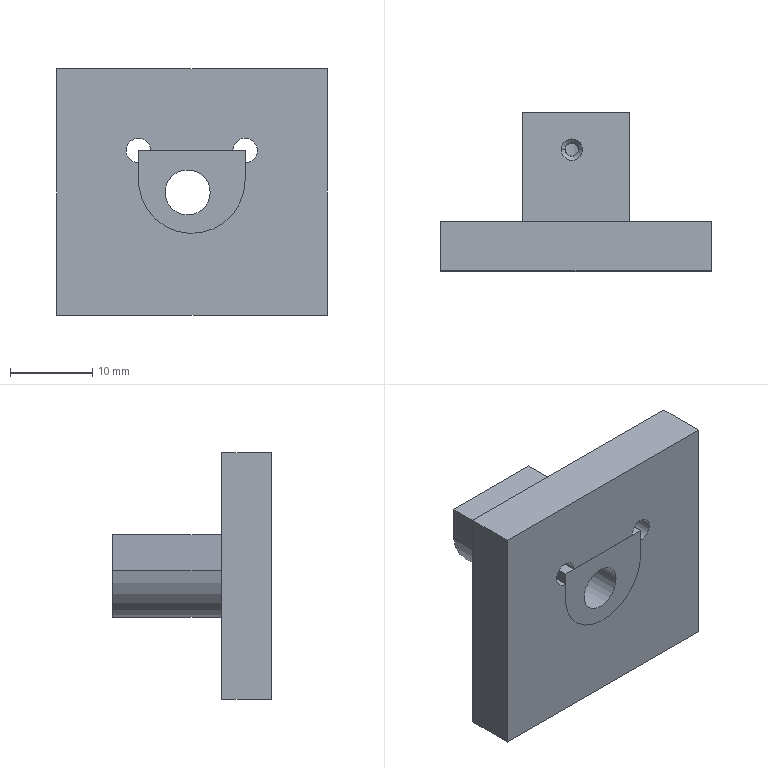NC program | NX | posted with a generic post | part box 32.951 x 19.3 x 30.1 mm
Lines 41 to 897 of 2866:
(ZLEVEL_PROFILE_COPY_1 , TOOL : D6)
N68 T06 M6
N70 G54
N72 G17 G0 G90 X-9.554 Y-0.868 B0. C0. S9500 M3
N74 G43 Z30. H6
N76 Z1.5
N78 G94 G1 X-9.55 Y-0.467 Z1.479 F1000.
N80 X-9.505 Y-0.031 Z1.456
N82 X-9.275 Y1.064 Z1.397
N84 X-8.921 Y2.124 Z1.339
N86 X-8.445 Y3.136 Z1.28
N88 X-7.855 Y4.086 Z1.222
N90 X-7.159 Y4.961 Z1.163
N92 X-6.365 Y5.75 Z1.104
N94 X-5.486 Y6.44 Z1.046
N96 X-4.532 Y7.024 Z0.987
N98 X-3.741 Y7.402 Z0.941
N100 X-2.577 Y7.808 Z0.877
N102 X-1.371 Y8.062 Z0.812
N104 X-0.143 Y8.159 Z0.747
N106 X1.088 Y8.098 Z0.683
N108 X2.301 Y7.88 Z0.618
N110 X3.476 Y7.509 Z0.554
N112 X4.595 Y6.991 Z0.489
N114 X5.637 Y6.333 Z0.424
N116 X6.587 Y5.548 Z0.36
N118 X7.428 Y4.647 Z0.295
N120 X8.147 Y3.646 Z0.231
N122 X8.733 Y2.562 Z0.166
N124 X9.174 Y1.411 Z0.101
N126 X9.465 Y0.213 Z0.037
N128 X9.6 Y-1.012 Z-0.028
N130 Y-5.299 Z-0.252
N132 X9.487 Y-5.915 Z-0.285
N134 X9.254 Y-6.495 Z-0.318
N136 X8.909 Y-7.017 Z-0.351
N138 X8.467 Y-7.459 Z-0.384
N140 X7.945 Y-7.804 Z-0.416
N142 X7.365 Y-8.037 Z-0.449
N144 X6.749 Y-8.15 Z-0.482
N146 X6.5 Z-0.495
N148 X-6.5 F2500.
N150 G2 X-9.6 Y-5.009 R3.1
N152 G1 X-9.55 Y-0.467
N154 G2 X9.6 Y-1.45 R9.6
N156 G1 Y-5.05
N158 G2 X6.5 Y-8.15 R3.1
N160 G1 X-6.293 Z-0.718
N162 X-6.465 Z-0.721
N164 X-6.638 Y-8.147 Z-0.724
N166 X-6.811 Y-8.134 Z-0.727
N168 X-6.982 Y-8.112 Z-0.73
N170 X-7.152 Y-8.081 Z-0.733
N172 X-7.32 Y-8.04 Z-0.736
N174 X-7.485 Y-7.989 Z-0.739
N176 X-7.648 Y-7.93 Z-0.742
N178 X-7.806 Y-7.861 Z-0.745
N180 X-7.961 Y-7.784 Z-0.748
N182 X-8.111 Y-7.698 Z-0.751
N184 X-8.256 Y-7.605 Z-0.754
N186 X-8.396 Y-7.503 Z-0.757
N188 X-8.53 Y-7.393 Z-0.76
N190 X-8.657 Y-7.276 Z-0.763
N192 X-8.778 Y-7.153 Z-0.767
N194 X-8.891 Y-7.023 Z-0.77
N196 X-8.998 Y-6.886 Z-0.773
N198 X-9.096 Y-6.744 Z-0.776
N200 X-9.187 Y-6.597 Z-0.779
N202 X-9.269 Y-6.445 Z-0.782
N204 X-9.342 Y-6.288 Z-0.785
N206 X-9.407 Y-6.128 Z-0.788
N208 X-9.462 Y-5.964 Z-0.791
N210 X-9.509 Y-5.798 Z-0.794
N212 X-9.545 Y-5.629 Z-0.797
N214 X-9.573 Y-5.458 Z-0.8
N216 X-9.591 Y-5.286 Z-0.803
N218 X-9.599 Y-5.114 Z-0.806
N220 Y-4.941 Z-0.809
N222 X-9.553 Y-0.792 Z-0.881
N224 X-9.551 Y-0.619 Z-0.884
N226 X-9.544 Y-0.447 Z-0.887
N228 X-9.528 Y-0.275 Z-0.89
N230 X-9.505 Y-0.103 Z-0.893
N232 X-9.479 Y0.068 Z-0.896
N234 X-9.45 Y0.238 Z-0.899
N236 X-9.418 Y0.408 Z-0.902
N238 X-9.383 Y0.577 Z-0.905
N240 X-9.345 Y0.746 Z-0.908
N242 X-9.304 Y0.914 Z-0.911
N244 X-9.26 Y1.081 Z-0.914
N246 X-9.213 Y1.247 Z-0.917
N248 X-9.163 Y1.413 Z-0.92
N250 X-9.11 Y1.577 Z-0.923
N252 X-9.054 Y1.741 Z-0.926
N254 X-8.995 Y1.903 Z-0.929
N256 X-8.933 Y2.065 Z-0.932
N258 X-8.869 Y2.225 Z-0.935
N260 X-8.801 Y2.384 Z-0.939
N262 X-8.731 Y2.542 Z-0.942
N264 X-8.657 Y2.699 Z-0.945
N266 X-8.581 Y2.854 Z-0.948
N268 X-8.502 Y3.008 Z-0.951
N270 X-8.421 Y3.16 Z-0.954
N272 X-8.336 Y3.311 Z-0.957
N274 X-8.249 Y3.46 Z-0.96
N276 X-8.159 Y3.608 Z-0.963
N278 X-8.067 Y3.754 Z-0.966
N280 X-7.972 Y3.899 Z-0.969
N282 X-7.874 Y4.041 Z-0.972
N284 X-7.774 Y4.182 Z-0.975
N286 X-7.672 Y4.321 Z-0.978
N288 X-7.566 Y4.458 Z-0.981
N290 X-7.459 Y4.594 Z-0.984
N292 X-7.349 Y4.727 Z-0.987
N294 X-7.236 Y4.858 Z-0.99
N296 G2 X9.6 Y-1.45 R9.6
N298 G1 Y-5.05
N300 G2 X6.5 Y-8.15 R3.1
N302 G1 X-6.293 Z-1.213
N304 X-6.465 Z-1.216
N306 X-6.638 Y-8.147 Z-1.219
N308 X-6.811 Y-8.134 Z-1.222
N310 X-6.982 Y-8.112 Z-1.225
N312 X-7.152 Y-8.081 Z-1.228
N314 X-7.32 Y-8.04 Z-1.231
N316 X-7.485 Y-7.989 Z-1.234
N318 X-7.648 Y-7.93 Z-1.237
N320 X-7.806 Y-7.861 Z-1.24
N322 X-7.961 Y-7.784 Z-1.243
N324 X-8.111 Y-7.698 Z-1.246
N326 X-8.256 Y-7.605 Z-1.249
N328 X-8.396 Y-7.503 Z-1.252
N330 X-8.53 Y-7.393 Z-1.255
N332 X-8.657 Y-7.276 Z-1.258
N334 X-8.778 Y-7.153 Z-1.261
N336 X-8.891 Y-7.023 Z-1.264
N338 X-8.998 Y-6.886 Z-1.267
N340 X-9.096 Y-6.744 Z-1.27
N342 X-9.187 Y-6.597 Z-1.273
N344 X-9.269 Y-6.445 Z-1.276
N346 X-9.342 Y-6.288 Z-1.279
N348 X-9.407 Y-6.128 Z-1.283
N350 X-9.462 Y-5.964 Z-1.286
N352 X-9.509 Y-5.798 Z-1.289
N354 X-9.545 Y-5.629 Z-1.292
N356 X-9.573 Y-5.458 Z-1.295
N358 X-9.591 Y-5.286 Z-1.298
N360 X-9.599 Y-5.114 Z-1.301
N362 Y-4.941 Z-1.304
N364 X-9.553 Y-0.792 Z-1.376
N366 X-9.551 Y-0.619 Z-1.379
N368 X-9.544 Y-0.447 Z-1.382
N370 X-9.528 Y-0.275 Z-1.385
N372 X-9.505 Y-0.103 Z-1.388
N374 X-9.479 Y0.068 Z-1.391
N376 X-9.45 Y0.238 Z-1.394
N378 X-9.418 Y0.408 Z-1.397
N380 X-9.383 Y0.577 Z-1.4
N382 X-9.345 Y0.746 Z-1.403
N384 X-9.304 Y0.914 Z-1.406
N386 X-9.26 Y1.081 Z-1.409
N388 X-9.213 Y1.247 Z-1.412
N390 X-9.163 Y1.413 Z-1.415
N392 X-9.11 Y1.577 Z-1.418
N394 X-9.054 Y1.741 Z-1.421
N396 X-8.995 Y1.903 Z-1.424
N398 X-8.933 Y2.065 Z-1.427
N400 X-8.869 Y2.225 Z-1.43
N402 X-8.801 Y2.384 Z-1.433
N404 X-8.731 Y2.542 Z-1.436
N406 X-8.657 Y2.699 Z-1.439
N408 X-8.581 Y2.854 Z-1.442
N410 X-8.502 Y3.008 Z-1.445
N412 X-8.421 Y3.16 Z-1.448
N414 X-8.336 Y3.311 Z-1.451
N416 X-8.249 Y3.46 Z-1.455
N418 X-8.159 Y3.608 Z-1.458
N420 X-8.067 Y3.754 Z-1.461
N422 X-7.972 Y3.899 Z-1.464
N424 X-7.874 Y4.041 Z-1.467
N426 X-7.774 Y4.182 Z-1.47
N428 X-7.672 Y4.321 Z-1.473
N430 X-7.566 Y4.458 Z-1.476
N432 X-7.459 Y4.594 Z-1.479
N434 X-7.349 Y4.727 Z-1.482
N436 X-7.236 Y4.858 Z-1.485
N438 G2 X9.6 Y-1.45 R9.6
N440 G1 Y-5.05
N442 G2 X6.5 Y-8.15 R3.1
N444 G1 X-6.293 Z-1.708
N446 X-6.465 Z-1.711
N448 X-6.638 Y-8.147 Z-1.714
N450 X-6.811 Y-8.134 Z-1.717
N452 X-6.982 Y-8.112 Z-1.72
N454 X-7.152 Y-8.081 Z-1.723
N456 X-7.32 Y-8.04 Z-1.726
N458 X-7.485 Y-7.989 Z-1.729
N460 X-7.648 Y-7.93 Z-1.732
N462 X-7.806 Y-7.861 Z-1.735
N464 X-7.961 Y-7.784 Z-1.738
N466 X-8.111 Y-7.698 Z-1.741
N468 X-8.256 Y-7.605 Z-1.744
N470 X-8.396 Y-7.503 Z-1.747
N472 X-8.53 Y-7.393 Z-1.75
N474 X-8.657 Y-7.276 Z-1.753
N476 X-8.778 Y-7.153 Z-1.756
N478 X-8.891 Y-7.023 Z-1.759
N480 X-8.998 Y-6.886 Z-1.762
N482 X-9.096 Y-6.744 Z-1.765
N484 X-9.187 Y-6.597 Z-1.768
N486 X-9.269 Y-6.445 Z-1.771
N488 X-9.342 Y-6.288 Z-1.774
N490 X-9.407 Y-6.128 Z-1.777
N492 X-9.462 Y-5.964 Z-1.78
N494 X-9.509 Y-5.798 Z-1.783
N496 X-9.545 Y-5.629 Z-1.786
N498 X-9.573 Y-5.458 Z-1.789
N500 X-9.591 Y-5.286 Z-1.792
N502 X-9.599 Y-5.114 Z-1.795
N504 Y-4.941 Z-1.799
N506 X-9.553 Y-0.792 Z-1.871
N508 X-9.551 Y-0.619 Z-1.874
N510 X-9.544 Y-0.447 Z-1.877
N512 X-9.528 Y-0.275 Z-1.88
N514 X-9.505 Y-0.103 Z-1.883
N516 X-9.479 Y0.068 Z-1.886
N518 X-9.45 Y0.238 Z-1.889
N520 X-9.418 Y0.408 Z-1.892
N522 X-9.383 Y0.577 Z-1.895
N524 X-9.345 Y0.746 Z-1.898
N526 X-9.304 Y0.914 Z-1.901
N528 X-9.26 Y1.081 Z-1.904
N530 X-9.213 Y1.247 Z-1.907
N532 X-9.163 Y1.413 Z-1.91
N534 X-9.11 Y1.577 Z-1.913
N536 X-9.054 Y1.741 Z-1.916
N538 X-8.995 Y1.903 Z-1.919
N540 X-8.933 Y2.065 Z-1.922
N542 X-8.869 Y2.225 Z-1.925
N544 X-8.801 Y2.384 Z-1.928
N546 X-8.731 Y2.542 Z-1.931
N548 X-8.657 Y2.699 Z-1.934
N550 X-8.581 Y2.854 Z-1.937
N552 X-8.502 Y3.008 Z-1.94
N554 X-8.421 Y3.16 Z-1.943
N556 X-8.336 Y3.311 Z-1.946
N558 X-8.249 Y3.46 Z-1.949
N560 X-8.159 Y3.608 Z-1.952
N562 X-8.067 Y3.754 Z-1.955
N564 X-7.972 Y3.899 Z-1.958
N566 X-7.874 Y4.041 Z-1.961
N568 X-7.774 Y4.182 Z-1.964
N570 X-7.672 Y4.321 Z-1.967
N572 X-7.566 Y4.458 Z-1.971
N574 X-7.459 Y4.594 Z-1.974
N576 X-7.349 Y4.727 Z-1.977
N578 X-7.236 Y4.858 Z-1.98
N580 G2 X9.6 Y-1.45 R9.6
N582 G1 Y-5.05
N584 G2 X6.5 Y-8.15 R3.1
N586 G1 X-6.293 Z-2.203
N588 X-6.465 Z-2.206
N590 X-6.638 Y-8.147 Z-2.209
N592 X-6.811 Y-8.134 Z-2.212
N594 X-6.982 Y-8.112 Z-2.215
N596 X-7.152 Y-8.081 Z-2.218
N598 X-7.32 Y-8.04 Z-2.221
N600 X-7.485 Y-7.989 Z-2.224
N602 X-7.648 Y-7.93 Z-2.227
N604 X-7.806 Y-7.861 Z-2.23
N606 X-7.961 Y-7.784 Z-2.233
N608 X-8.111 Y-7.698 Z-2.236
N610 X-8.256 Y-7.605 Z-2.239
N612 X-8.396 Y-7.503 Z-2.242
N614 X-8.53 Y-7.393 Z-2.245
N616 X-8.657 Y-7.276 Z-2.248
N618 X-8.778 Y-7.153 Z-2.251
N620 X-8.891 Y-7.023 Z-2.254
N622 X-8.998 Y-6.886 Z-2.257
N624 X-9.096 Y-6.744 Z-2.26
N626 X-9.187 Y-6.597 Z-2.263
N628 X-9.269 Y-6.445 Z-2.266
N630 X-9.342 Y-6.288 Z-2.269
N632 X-9.407 Y-6.128 Z-2.272
N634 X-9.462 Y-5.964 Z-2.275
N636 X-9.509 Y-5.798 Z-2.278
N638 X-9.545 Y-5.629 Z-2.281
N640 X-9.573 Y-5.458 Z-2.284
N642 X-9.591 Y-5.286 Z-2.287
N644 X-9.599 Y-5.114 Z-2.29
N646 Y-4.941 Z-2.293
N648 X-9.553 Y-0.792 Z-2.366
N650 X-9.551 Y-0.619 Z-2.369
N652 X-9.544 Y-0.447 Z-2.372
N654 X-9.528 Y-0.275 Z-2.375
N656 X-9.505 Y-0.103 Z-2.378
N658 X-9.479 Y0.068 Z-2.381
N660 X-9.45 Y0.238 Z-2.384
N662 X-9.418 Y0.408 Z-2.387
N664 X-9.383 Y0.577 Z-2.39
N666 X-9.345 Y0.746 Z-2.393
N668 X-9.304 Y0.914 Z-2.396
N670 X-9.26 Y1.081 Z-2.399
N672 X-9.213 Y1.247 Z-2.402
N674 X-9.163 Y1.413 Z-2.405
N676 X-9.11 Y1.577 Z-2.408
N678 X-9.054 Y1.741 Z-2.411
N680 X-8.995 Y1.903 Z-2.414
N682 X-8.933 Y2.065 Z-2.417
N684 X-8.869 Y2.225 Z-2.42
N686 X-8.801 Y2.384 Z-2.423
N688 X-8.731 Y2.542 Z-2.426
N690 X-8.657 Y2.699 Z-2.429
N692 X-8.581 Y2.854 Z-2.432
N694 X-8.502 Y3.008 Z-2.435
N696 X-8.421 Y3.16 Z-2.438
N698 X-8.336 Y3.311 Z-2.441
N700 X-8.249 Y3.46 Z-2.444
N702 X-8.159 Y3.608 Z-2.447
N704 X-8.067 Y3.754 Z-2.45
N706 X-7.972 Y3.899 Z-2.453
N708 X-7.874 Y4.041 Z-2.456
N710 X-7.774 Y4.182 Z-2.459
N712 X-7.672 Y4.321 Z-2.462
N714 X-7.566 Y4.458 Z-2.465
N716 X-7.459 Y4.594 Z-2.468
N718 X-7.349 Y4.727 Z-2.471
N720 X-7.236 Y4.858 Z-2.474
N722 G2 X9.6 Y-1.45 R9.6
N724 G1 Y-5.05
N726 G2 X6.5 Y-8.15 R3.1
N728 G1 X-6.293 Z-2.698
N730 X-6.465 Z-2.701
N732 X-6.638 Y-8.147 Z-2.704
N734 X-6.811 Y-8.134 Z-2.707
N736 X-6.982 Y-8.112 Z-2.71
N738 X-7.152 Y-8.081 Z-2.713
N740 X-7.32 Y-8.04 Z-2.716
N742 X-7.485 Y-7.989 Z-2.719
N744 X-7.648 Y-7.93 Z-2.722
N746 X-7.806 Y-7.861 Z-2.725
N748 X-7.961 Y-7.784 Z-2.728
N750 X-8.111 Y-7.698 Z-2.731
N752 X-8.256 Y-7.605 Z-2.734
N754 X-8.396 Y-7.503 Z-2.737
N756 X-8.53 Y-7.393 Z-2.74
N758 X-8.657 Y-7.276 Z-2.743
N760 X-8.778 Y-7.153 Z-2.746
N762 X-8.891 Y-7.023 Z-2.749
N764 X-8.998 Y-6.886 Z-2.752
N766 X-9.096 Y-6.744 Z-2.755
N768 X-9.187 Y-6.597 Z-2.758
N770 X-9.269 Y-6.445 Z-2.761
N772 X-9.342 Y-6.288 Z-2.764
N774 X-9.407 Y-6.128 Z-2.767
N776 X-9.462 Y-5.964 Z-2.77
N778 X-9.509 Y-5.798 Z-2.773
N780 X-9.545 Y-5.629 Z-2.776
N782 X-9.573 Y-5.458 Z-2.779
N784 X-9.591 Y-5.286 Z-2.782
N786 X-9.599 Y-5.114 Z-2.785
N788 Y-4.941 Z-2.788
N790 X-9.553 Y-0.792 Z-2.861
N792 X-9.551 Y-0.619 Z-2.864
N794 X-9.544 Y-0.447 Z-2.867
N796 X-9.528 Y-0.275 Z-2.87
N798 X-9.505 Y-0.103 Z-2.873
N800 X-9.479 Y0.068 Z-2.876
N802 X-9.45 Y0.238 Z-2.879
N804 X-9.418 Y0.408 Z-2.882
N806 X-9.383 Y0.577 Z-2.885
N808 X-9.345 Y0.746 Z-2.888
N810 X-9.304 Y0.914 Z-2.891
N812 X-9.26 Y1.081 Z-2.894
N814 X-9.213 Y1.247 Z-2.897
N816 X-9.163 Y1.413 Z-2.9
N818 X-9.11 Y1.577 Z-2.903
N820 X-9.054 Y1.741 Z-2.906
N822 X-8.995 Y1.903 Z-2.909
N824 X-8.933 Y2.065 Z-2.912
N826 X-8.869 Y2.225 Z-2.915
N828 X-8.801 Y2.384 Z-2.918
N830 X-8.731 Y2.542 Z-2.921
N832 X-8.657 Y2.699 Z-2.924
N834 X-8.581 Y2.854 Z-2.927
N836 X-8.502 Y3.008 Z-2.93
N838 X-8.421 Y3.16 Z-2.933
N840 X-8.336 Y3.311 Z-2.936
N842 X-8.249 Y3.46 Z-2.939
N844 X-8.159 Y3.608 Z-2.942
N846 X-8.067 Y3.754 Z-2.945
N848 X-7.972 Y3.899 Z-2.948
N850 X-7.874 Y4.041 Z-2.951
N852 X-7.774 Y4.182 Z-2.954
N854 X-7.672 Y4.321 Z-2.957
N856 X-7.566 Y4.458 Z-2.96
N858 X-7.459 Y4.594 Z-2.963
N860 X-7.349 Y4.727 Z-2.966
N862 X-7.236 Y4.858 Z-2.969
N864 G2 X9.6 Y-1.45 R9.6
N866 G1 Y-5.05
N868 G2 X6.5 Y-8.15 R3.1
N870 G1 X-6.293 Z-3.193
N872 X-6.465 Z-3.196
N874 X-6.638 Y-8.147 Z-3.199
N876 X-6.811 Y-8.134 Z-3.202
N878 X-6.982 Y-8.112 Z-3.205
N880 X-7.152 Y-8.081 Z-3.208
N882 X-7.32 Y-8.04 Z-3.211
N884 X-7.485 Y-7.989 Z-3.214
N886 X-7.648 Y-7.93 Z-3.217
N888 X-7.806 Y-7.861 Z-3.22
N890 X-7.961 Y-7.784 Z-3.223
N892 X-8.111 Y-7.698 Z-3.226
N894 X-8.256 Y-7.605 Z-3.229
N896 X-8.396 Y-7.503 Z-3.232
N898 X-8.53 Y-7.393 Z-3.235
N900 X-8.657 Y-7.276 Z-3.238
N902 X-8.778 Y-7.153 Z-3.241
N904 X-8.891 Y-7.023 Z-3.244
N906 X-8.998 Y-6.886 Z-3.247
N908 X-9.096 Y-6.744 Z-3.25
N910 X-9.187 Y-6.597 Z-3.253
N912 X-9.269 Y-6.445 Z-3.256
N914 X-9.342 Y-6.288 Z-3.259
N916 X-9.407 Y-6.128 Z-3.262
N918 X-9.462 Y-5.964 Z-3.265
N920 X-9.509 Y-5.798 Z-3.268
N922 X-9.545 Y-5.629 Z-3.271
N924 X-9.573 Y-5.458 Z-3.274
N926 X-9.591 Y-5.286 Z-3.277
N928 X-9.599 Y-5.114 Z-3.28
N930 Y-4.941 Z-3.283
N932 X-9.553 Y-0.792 Z-3.356
N934 X-9.551 Y-0.619 Z-3.359
N936 X-9.544 Y-0.447 Z-3.362
N938 X-9.528 Y-0.275 Z-3.365
N940 X-9.505 Y-0.103 Z-3.368
N942 X-9.479 Y0.068 Z-3.371
N944 X-9.45 Y0.238 Z-3.374
N946 X-9.418 Y0.408 Z-3.377
N948 X-9.383 Y0.577 Z-3.38
N950 X-9.345 Y0.746 Z-3.383
N952 X-9.304 Y0.914 Z-3.386
N954 X-9.26 Y1.081 Z-3.389
N956 X-9.213 Y1.247 Z-3.392
N958 X-9.163 Y1.413 Z-3.395
N960 X-9.11 Y1.577 Z-3.398
N962 X-9.054 Y1.741 Z-3.401
N964 X-8.995 Y1.903 Z-3.404
N966 X-8.933 Y2.065 Z-3.407
N968 X-8.869 Y2.225 Z-3.41
N970 X-8.801 Y2.384 Z-3.413
N972 X-8.731 Y2.542 Z-3.416
N974 X-8.657 Y2.699 Z-3.419
N976 X-8.581 Y2.854 Z-3.422
N978 X-8.502 Y3.008 Z-3.425
N980 X-8.421 Y3.16 Z-3.428
N982 X-8.336 Y3.311 Z-3.431
N984 X-8.249 Y3.46 Z-3.434
N986 X-8.159 Y3.608 Z-3.437
N988 X-8.067 Y3.754 Z-3.44
N990 X-7.972 Y3.899 Z-3.443
N992 X-7.874 Y4.041 Z-3.446
N994 X-7.774 Y4.182 Z-3.449
N996 X-7.672 Y4.321 Z-3.452
N998 X-7.566 Y4.458 Z-3.455
N1000 X-7.459 Y4.594 Z-3.458
N1002 X-7.349 Y4.727 Z-3.461
N1004 X-7.236 Y4.858 Z-3.464
N1006 G2 X9.6 Y-1.45 R9.6
N1008 G1 Y-5.05
N1010 G2 X6.5 Y-8.15 R3.1
N1012 G1 X-6.293 Z-3.687
N1014 X-6.465 Z-3.69
N1016 X-6.638 Y-8.147 Z-3.694
N1018 X-6.811 Y-8.134 Z-3.697
N1020 X-6.982 Y-8.112 Z-3.7
N1022 X-7.152 Y-8.081 Z-3.703
N1024 X-7.32 Y-8.04 Z-3.706
N1026 X-7.485 Y-7.989 Z-3.709
N1028 X-7.648 Y-7.93 Z-3.712
N1030 X-7.806 Y-7.861 Z-3.715
N1032 X-7.961 Y-7.784 Z-3.718
N1034 X-8.111 Y-7.698 Z-3.721
N1036 X-8.256 Y-7.605 Z-3.724
N1038 X-8.396 Y-7.503 Z-3.727
N1040 X-8.53 Y-7.393 Z-3.73
N1042 X-8.657 Y-7.276 Z-3.733
N1044 X-8.778 Y-7.153 Z-3.736
N1046 X-8.891 Y-7.023 Z-3.739
N1048 X-8.998 Y-6.886 Z-3.742
N1050 X-9.096 Y-6.744 Z-3.745
N1052 X-9.187 Y-6.597 Z-3.748
N1054 X-9.269 Y-6.445 Z-3.751
N1056 X-9.342 Y-6.288 Z-3.754
N1058 X-9.407 Y-6.128 Z-3.757
N1060 X-9.462 Y-5.964 Z-3.76
N1062 X-9.509 Y-5.798 Z-3.763
N1064 X-9.545 Y-5.629 Z-3.766
N1066 X-9.573 Y-5.458 Z-3.769
N1068 X-9.591 Y-5.286 Z-3.772
N1070 X-9.599 Y-5.114 Z-3.775
N1072 Y-4.941 Z-3.778
N1074 X-9.553 Y-0.792 Z-3.85
N1076 X-9.551 Y-0.619 Z-3.853
N1078 X-9.544 Y-0.447 Z-3.856
N1080 X-9.528 Y-0.275 Z-3.859
N1082 X-9.505 Y-0.103 Z-3.862
N1084 X-9.479 Y0.068 Z-3.865
N1086 X-9.45 Y0.238 Z-3.869
N1088 X-9.418 Y0.408 Z-3.872
N1090 X-9.383 Y0.577 Z-3.875
N1092 X-9.345 Y0.746 Z-3.878
N1094 X-9.304 Y0.914 Z-3.881
N1096 X-9.26 Y1.081 Z-3.884
N1098 X-9.213 Y1.247 Z-3.887
N1100 X-9.163 Y1.413 Z-3.89
N1102 X-9.11 Y1.577 Z-3.893
N1104 X-9.054 Y1.741 Z-3.896
N1106 X-8.995 Y1.903 Z-3.899
N1108 X-8.933 Y2.065 Z-3.902
N1110 X-8.869 Y2.225 Z-3.905
N1112 X-8.801 Y2.384 Z-3.908
N1114 X-8.731 Y2.542 Z-3.911
N1116 X-8.657 Y2.699 Z-3.914
N1118 X-8.581 Y2.854 Z-3.917
N1120 X-8.502 Y3.008 Z-3.92
N1122 X-8.421 Y3.16 Z-3.923
N1124 X-8.336 Y3.311 Z-3.926
N1126 X-8.249 Y3.46 Z-3.929
N1128 X-8.159 Y3.608 Z-3.932
N1130 X-8.067 Y3.754 Z-3.935
N1132 X-7.972 Y3.899 Z-3.938
N1134 X-7.874 Y4.041 Z-3.941
N1136 X-7.774 Y4.182 Z-3.944
N1138 X-7.672 Y4.321 Z-3.947
N1140 X-7.566 Y4.458 Z-3.95
N1142 X-7.459 Y4.594 Z-3.953
N1144 X-7.349 Y4.727 Z-3.956
N1146 X-7.236 Y4.858 Z-3.959
N1148 G2 X9.6 Y-1.45 R9.6
N1150 G1 Y-5.05
N1152 G2 X6.5 Y-8.15 R3.1
N1154 G1 X-6.293 Z-4.182
N1156 X-6.465 Z-4.185
N1158 X-6.638 Y-8.147 Z-4.188
N1160 X-6.811 Y-8.134 Z-4.191
N1162 X-6.982 Y-8.112 Z-4.194
N1164 X-7.152 Y-8.081 Z-4.197
N1166 X-7.32 Y-8.04 Z-4.2
N1168 X-7.485 Y-7.989 Z-4.203
N1170 X-7.648 Y-7.93 Z-4.206
N1172 X-7.806 Y-7.861 Z-4.209
N1174 X-7.961 Y-7.784 Z-4.213
N1176 X-8.111 Y-7.698 Z-4.216
N1178 X-8.256 Y-7.605 Z-4.219
N1180 X-8.396 Y-7.503 Z-4.222
N1182 X-8.53 Y-7.393 Z-4.225
N1184 X-8.657 Y-7.276 Z-4.228
N1186 X-8.778 Y-7.153 Z-4.231
N1188 X-8.891 Y-7.023 Z-4.234
N1190 X-8.998 Y-6.886 Z-4.237
N1192 X-9.096 Y-6.744 Z-4.24
N1194 X-9.187 Y-6.597 Z-4.243
N1196 X-9.269 Y-6.445 Z-4.246
N1198 X-9.342 Y-6.288 Z-4.249
N1200 X-9.407 Y-6.128 Z-4.252
N1202 X-9.462 Y-5.964 Z-4.255
N1204 X-9.509 Y-5.798 Z-4.258
N1206 X-9.545 Y-5.629 Z-4.261
N1208 X-9.573 Y-5.458 Z-4.264
N1210 X-9.591 Y-5.286 Z-4.267
N1212 X-9.599 Y-5.114 Z-4.27
N1214 Y-4.941 Z-4.273
N1216 X-9.553 Y-0.792 Z-4.345
N1218 X-9.551 Y-0.619 Z-4.348
N1220 X-9.544 Y-0.447 Z-4.351
N1222 X-9.528 Y-0.275 Z-4.354
N1224 X-9.505 Y-0.103 Z-4.357
N1226 X-9.479 Y0.068 Z-4.36
N1228 X-9.45 Y0.238 Z-4.363
N1230 X-9.418 Y0.408 Z-4.366
N1232 X-9.383 Y0.577 Z-4.369
N1234 X-9.345 Y0.746 Z-4.372
N1236 X-9.304 Y0.914 Z-4.375
N1238 X-9.26 Y1.081 Z-4.378
N1240 X-9.213 Y1.247 Z-4.381
N1242 X-9.163 Y1.413 Z-4.385
N1244 X-9.11 Y1.577 Z-4.388
N1246 X-9.054 Y1.741 Z-4.391
N1248 X-8.995 Y1.903 Z-4.394
N1250 X-8.933 Y2.065 Z-4.397
N1252 X-8.869 Y2.225 Z-4.4
N1254 X-8.801 Y2.384 Z-4.403
N1256 X-8.731 Y2.542 Z-4.406
N1258 X-8.657 Y2.699 Z-4.409
N1260 X-8.581 Y2.854 Z-4.412
N1262 X-8.502 Y3.008 Z-4.415
N1264 X-8.421 Y3.16 Z-4.418
N1266 X-8.336 Y3.311 Z-4.421
N1268 X-8.249 Y3.46 Z-4.424
N1270 X-8.159 Y3.608 Z-4.427
N1272 X-8.067 Y3.754 Z-4.43
N1274 X-7.972 Y3.899 Z-4.433
N1276 X-7.874 Y4.041 Z-4.436
N1278 X-7.774 Y4.182 Z-4.439
N1280 X-7.672 Y4.321 Z-4.442
N1282 X-7.566 Y4.458 Z-4.445
N1284 X-7.459 Y4.594 Z-4.448
N1286 X-7.349 Y4.727 Z-4.451
N1288 X-7.236 Y4.858 Z-4.454
N1290 G2 X9.6 Y-1.45 R9.6
N1292 G1 Y-5.05
N1294 G2 X6.5 Y-8.15 R3.1
N1296 G1 X-6.293 Z-4.677
N1298 X-6.465 Z-4.68
N1300 X-6.638 Y-8.147 Z-4.683
N1302 X-6.811 Y-8.134 Z-4.686
N1304 X-6.982 Y-8.112 Z-4.689
N1306 X-7.152 Y-8.081 Z-4.692
N1308 X-7.32 Y-8.04 Z-4.695
N1310 X-7.485 Y-7.989 Z-4.698
N1312 X-7.648 Y-7.93 Z-4.701
N1314 X-7.806 Y-7.861 Z-4.704
N1316 X-7.961 Y-7.784 Z-4.707
N1318 X-8.111 Y-7.698 Z-4.71
N1320 X-8.256 Y-7.605 Z-4.713
N1322 X-8.396 Y-7.503 Z-4.716
N1324 X-8.53 Y-7.393 Z-4.719
N1326 X-8.657 Y-7.276 Z-4.722
N1328 X-8.778 Y-7.153 Z-4.725
N1330 X-8.891 Y-7.023 Z-4.729
N1332 X-8.998 Y-6.886 Z-4.732
N1334 X-9.096 Y-6.744 Z-4.735
N1336 X-9.187 Y-6.597 Z-4.738
N1338 X-9.269 Y-6.445 Z-4.741
N1340 X-9.342 Y-6.288 Z-4.744
N1342 X-9.407 Y-6.128 Z-4.747
N1344 X-9.462 Y-5.964 Z-4.75
N1346 X-9.509 Y-5.798 Z-4.753
N1348 X-9.545 Y-5.629 Z-4.756
N1350 X-9.573 Y-5.458 Z-4.759
N1352 X-9.591 Y-5.286 Z-4.762
N1354 X-9.599 Y-5.114 Z-4.765
N1356 Y-4.941 Z-4.768
N1358 X-9.553 Y-0.792 Z-4.84
N1360 X-9.551 Y-0.619 Z-4.843
N1362 X-9.544 Y-0.447 Z-4.846
N1364 X-9.528 Y-0.275 Z-4.849
N1366 X-9.505 Y-0.103 Z-4.852
N1368 X-9.479 Y0.068 Z-4.855
N1370 X-9.45 Y0.238 Z-4.858
N1372 X-9.418 Y0.408 Z-4.861
N1374 X-9.383 Y0.577 Z-4.864
N1376 X-9.345 Y0.746 Z-4.867
N1378 X-9.304 Y0.914 Z-4.87
N1380 X-9.26 Y1.081 Z-4.873
N1382 X-9.213 Y1.247 Z-4.876
N1384 X-9.163 Y1.413 Z-4.879
N1386 X-9.11 Y1.577 Z-4.882
N1388 X-9.054 Y1.741 Z-4.885
N1390 X-8.995 Y1.903 Z-4.888
N1392 X-8.933 Y2.065 Z-4.891
N1394 X-8.869 Y2.225 Z-4.894
N1396 X-8.801 Y2.384 Z-4.897
N1398 X-8.731 Y2.542 Z-4.901
N1400 X-8.657 Y2.699 Z-4.904
N1402 X-8.581 Y2.854 Z-4.907
N1404 X-8.502 Y3.008 Z-4.91
N1406 X-8.421 Y3.16 Z-4.913
N1408 X-8.336 Y3.311 Z-4.916
N1410 X-8.249 Y3.46 Z-4.919
N1412 X-8.159 Y3.608 Z-4.922
N1414 X-8.067 Y3.754 Z-4.925
N1416 X-7.972 Y3.899 Z-4.928
N1418 X-7.874 Y4.041 Z-4.931
N1420 X-7.774 Y4.182 Z-4.934
N1422 X-7.672 Y4.321 Z-4.937
N1424 X-7.566 Y4.458 Z-4.94
N1426 X-7.459 Y4.594 Z-4.943
N1428 X-7.349 Y4.727 Z-4.946
N1430 X-7.236 Y4.858 Z-4.949
N1432 G2 X9.6 Y-1.45 R9.6
N1434 G1 Y-5.05
N1436 G2 X6.5 Y-8.15 R3.1
N1438 G1 X-6.293 Z-5.172
N1440 X-6.465 Z-5.175
N1442 X-6.638 Y-8.147 Z-5.178
N1444 X-6.811 Y-8.134 Z-5.181
N1446 X-6.982 Y-8.112 Z-5.184
N1448 X-7.152 Y-8.081 Z-5.187
N1450 X-7.32 Y-8.04 Z-5.19
N1452 X-7.485 Y-7.989 Z-5.193
N1454 X-7.648 Y-7.93 Z-5.196
N1456 X-7.806 Y-7.861 Z-5.199
N1458 X-7.961 Y-7.784 Z-5.202
N1460 X-8.111 Y-7.698 Z-5.205
N1462 X-8.256 Y-7.605 Z-5.208
N1464 X-8.396 Y-7.503 Z-5.211
N1466 X-8.53 Y-7.393 Z-5.214
N1468 X-8.657 Y-7.276 Z-5.217
N1470 X-8.778 Y-7.153 Z-5.22
N1472 X-8.891 Y-7.023 Z-5.223
N1474 X-8.998 Y-6.886 Z-5.226
N1476 X-9.096 Y-6.744 Z-5.229
N1478 X-9.187 Y-6.597 Z-5.232
N1480 X-9.269 Y-6.445 Z-5.235
N1482 X-9.342 Y-6.288 Z-5.238
N1484 X-9.407 Y-6.128 Z-5.241
N1486 X-9.462 Y-5.964 Z-5.245
N1488 X-9.509 Y-5.798 Z-5.248
N1490 X-9.545 Y-5.629 Z-5.251
N1492 X-9.573 Y-5.458 Z-5.254
N1494 X-9.591 Y-5.286 Z-5.257
N1496 X-9.599 Y-5.114 Z-5.26
N1498 Y-4.941 Z-5.263
N1500 X-9.553 Y-0.792 Z-5.335
N1502 X-9.551 Y-0.619 Z-5.338
N1504 X-9.544 Y-0.447 Z-5.341
N1506 X-9.528 Y-0.275 Z-5.344
N1508 X-9.505 Y-0.103 Z-5.347
N1510 X-9.479 Y0.068 Z-5.35
N1512 X-9.45 Y0.238 Z-5.353
N1514 X-9.418 Y0.408 Z-5.356
N1516 X-9.383 Y0.577 Z-5.359
N1518 X-9.345 Y0.746 Z-5.362
N1520 X-9.304 Y0.914 Z-5.365
N1522 X-9.26 Y1.081 Z-5.368
N1524 X-9.213 Y1.247 Z-5.371
N1526 X-9.163 Y1.413 Z-5.374
N1528 X-9.11 Y1.577 Z-5.377
N1530 X-9.054 Y1.741 Z-5.38
N1532 X-8.995 Y1.903 Z-5.383
N1534 X-8.933 Y2.065 Z-5.386
N1536 X-8.869 Y2.225 Z-5.389
N1538 X-8.801 Y2.384 Z-5.392
N1540 X-8.731 Y2.542 Z-5.395
N1542 X-8.657 Y2.699 Z-5.398
N1544 X-8.581 Y2.854 Z-5.401
N1546 X-8.502 Y3.008 Z-5.404
N1548 X-8.421 Y3.16 Z-5.407
N1550 X-8.336 Y3.311 Z-5.41
N1552 X-8.249 Y3.46 Z-5.413
N1554 X-8.159 Y3.608 Z-5.416
N1556 X-8.067 Y3.754 Z-5.42
N1558 X-7.972 Y3.899 Z-5.423
N1560 X-7.874 Y4.041 Z-5.426
N1562 X-7.774 Y4.182 Z-5.429
N1564 X-7.672 Y4.321 Z-5.432
N1566 X-7.566 Y4.458 Z-5.435
N1568 X-7.459 Y4.594 Z-5.438
N1570 X-7.349 Y4.727 Z-5.441
N1572 X-7.236 Y4.858 Z-5.444
N1574 G2 X9.6 Y-1.45 R9.6
N1576 G1 Y-5.05
N1578 G2 X6.5 Y-8.15 R3.1
N1580 G1 X-6.293 Z-5.667
N1582 X-6.465 Z-5.67
N1584 X-6.638 Y-8.147 Z-5.673
N1586 X-6.811 Y-8.134 Z-5.676
N1588 X-6.982 Y-8.112 Z-5.679
N1590 X-7.152 Y-8.081 Z-5.682
N1592 X-7.32 Y-8.04 Z-5.685
N1594 X-7.485 Y-7.989 Z-5.688
N1596 X-7.648 Y-7.93 Z-5.691
N1598 X-7.806 Y-7.861 Z-5.694
N1600 X-7.961 Y-7.784 Z-5.697
N1602 X-8.111 Y-7.698 Z-5.7
N1604 X-8.256 Y-7.605 Z-5.703
N1606 X-8.396 Y-7.503 Z-5.706
N1608 X-8.53 Y-7.393 Z-5.709
N1610 X-8.657 Y-7.276 Z-5.712
N1612 X-8.778 Y-7.153 Z-5.715
N1614 X-8.891 Y-7.023 Z-5.718
N1616 X-8.998 Y-6.886 Z-5.721
N1618 X-9.096 Y-6.744 Z-5.724
N1620 X-9.187 Y-6.597 Z-5.727
N1622 X-9.269 Y-6.445 Z-5.73
N1624 X-9.342 Y-6.288 Z-5.733
N1626 X-9.407 Y-6.128 Z-5.736
N1628 X-9.462 Y-5.964 Z-5.739
N1630 X-9.509 Y-5.798 Z-5.742
N1632 X-9.545 Y-5.629 Z-5.745
N1634 X-9.573 Y-5.458 Z-5.748
N1636 X-9.591 Y-5.286 Z-5.751
N1638 X-9.599 Y-5.114 Z-5.754
N1640 Y-4.941 Z-5.757
N1642 X-9.553 Y-0.792 Z-5.83
N1644 X-9.551 Y-0.619 Z-5.833
N1646 X-9.544 Y-0.447 Z-5.836
N1648 X-9.528 Y-0.275 Z-5.839
N1650 X-9.505 Y-0.103 Z-5.842
N1652 X-9.479 Y0.068 Z-5.845
N1654 X-9.45 Y0.238 Z-5.848
N1656 X-9.418 Y0.408 Z-5.851
N1658 X-9.383 Y0.577 Z-5.854
N1660 X-9.345 Y0.746 Z-5.857
N1662 X-9.304 Y0.914 Z-5.86
N1664 X-9.26 Y1.081 Z-5.863
N1666 X-9.213 Y1.247 Z-5.866
N1668 X-9.163 Y1.413 Z-5.869
N1670 X-9.11 Y1.577 Z-5.872
N1672 X-9.054 Y1.741 Z-5.875
N1674 X-8.995 Y1.903 Z-5.878
N1676 X-8.933 Y2.065 Z-5.881
N1678 X-8.869 Y2.225 Z-5.884
N1680 X-8.801 Y2.384 Z-5.887
N1682 X-8.731 Y2.542 Z-5.89
N1684 X-8.657 Y2.699 Z-5.893
N1686 X-8.581 Y2.854 Z-5.896
N1688 X-8.502 Y3.008 Z-5.899
N1690 X-8.421 Y3.16 Z-5.902
N1692 X-8.336 Y3.311 Z-5.905
N1694 X-8.249 Y3.46 Z-5.908
N1696 X-8.159 Y3.608 Z-5.911
N1698 X-8.067 Y3.754 Z-5.914
N1700 X-7.972 Y3.899 Z-5.917
N1702 X-7.874 Y4.041 Z-5.92
N1704 X-7.774 Y4.182 Z-5.923
N1706 X-7.672 Y4.321 Z-5.926
N1708 X-7.566 Y4.458 Z-5.929
N1710 X-7.459 Y4.594 Z-5.932
N1712 X-7.349 Y4.727 Z-5.936
N1714 X-7.236 Y4.858 Z-5.939
N1716 G2 X9.6 Y-1.45 R9.6
N1718 G1 Y-5.05
N1720 G2 X6.5 Y-8.15 R3.1
N1722 G1 X-6.293 Z-6.162
N1724 X-6.465 Z-6.165
N1726 X-6.638 Y-8.147 Z-6.168
N1728 X-6.811 Y-8.134 Z-6.171
N1730 X-6.982 Y-8.112 Z-6.174
N1732 X-7.152 Y-8.081 Z-6.177
N1734 X-7.32 Y-8.04 Z-6.18
N1736 X-7.485 Y-7.989 Z-6.183
N1738 X-7.648 Y-7.93 Z-6.186
N1740 X-7.806 Y-7.861 Z-6.189
N1742 X-7.961 Y-7.784 Z-6.192
N1744 X-8.111 Y-7.698 Z-6.195
N1746 X-8.256 Y-7.605 Z-6.198
N1748 X-8.396 Y-7.503 Z-6.201
N1750 X-8.53 Y-7.393 Z-6.204
N1752 X-8.657 Y-7.276 Z-6.207
N1754 X-8.778 Y-7.153 Z-6.21
N1756 X-8.891 Y-7.023 Z-6.213
N1758 X-8.998 Y-6.886 Z-6.216
N1760 X-9.096 Y-6.744 Z-6.219
N1762 X-9.187 Y-6.597 Z-6.222
N1764 X-9.269 Y-6.445 Z-6.225
N1766 X-9.342 Y-6.288 Z-6.228
N1768 X-9.407 Y-6.128 Z-6.231
N1770 X-9.462 Y-5.964 Z-6.234
N1772 X-9.509 Y-5.798 Z-6.237
N1774 X-9.545 Y-5.629 Z-6.24